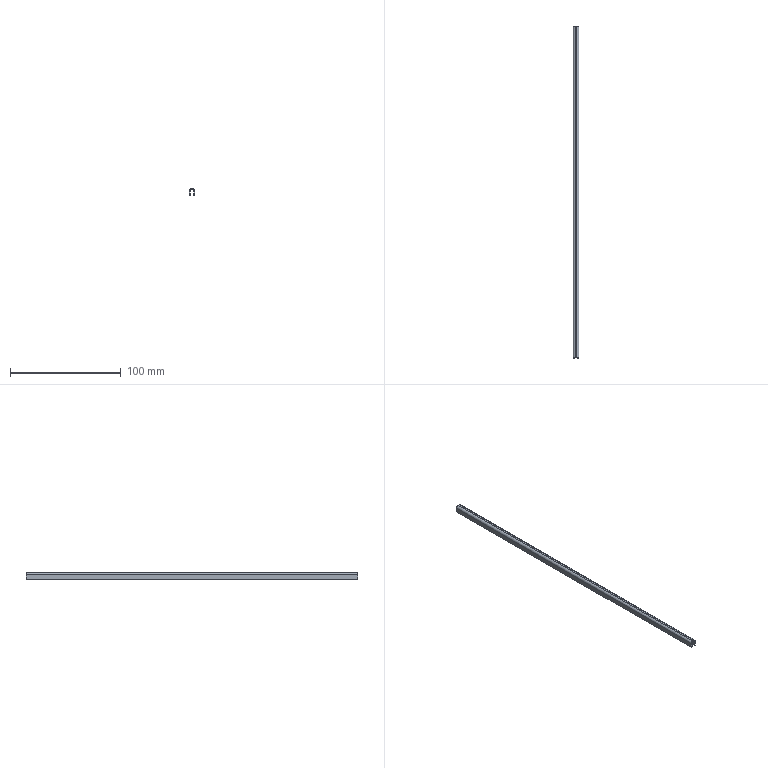Part | STEP file | Guide wheel mechanism revised.sldasm-Part-332 | 1 solid | 22 faces | box 5.4 x 300 x 6.2 mm | volume 5131 mm3 | plane 18 | cylinder 4 | commonest cylinder face diameters 1.473 x2 3.873 x2
STEP:
#1=CARTESIAN_POINT('',(-1.2,300.,-5.));
#2=VERTEX_POINT('',#1);
#3=CARTESIAN_POINT('',(-1.2,0.,-5.));
#4=VERTEX_POINT('',#3);
#5=CARTESIAN_POINT('',(-1.2,300.,-5.));
#6=DIRECTION('',(0.,-1.,0.));
#7=VECTOR('',#6,1000.);
#8=LINE('',#5,#7);
#9=EDGE_CURVE('',#2,#4,#8,.T.);
#10=ORIENTED_EDGE('',*,*,#9,.F.);
#11=CARTESIAN_POINT('',(0.,300.,-5.));
#12=VERTEX_POINT('',#11);
#13=CARTESIAN_POINT('',(598.861,300.,-5.));
#14=DIRECTION('',(-1.,0.,0.));
#15=VECTOR('',#14,1000.);
#16=LINE('',#13,#15);
#17=EDGE_CURVE('',#12,#2,#16,.T.);
#18=ORIENTED_EDGE('',*,*,#17,.F.);
#19=CARTESIAN_POINT('',(0.,0.,-5.));
#20=VERTEX_POINT('',#19);
#21=CARTESIAN_POINT('',(0.,300.,-5.));
#22=DIRECTION('',(0.,-1.,0.));
#23=VECTOR('',#22,1000.);
#24=LINE('',#21,#23);
#25=EDGE_CURVE('',#12,#20,#24,.T.);
#26=ORIENTED_EDGE('',*,*,#25,.T.);
#27=CARTESIAN_POINT('',(598.861,0.,-5.));
#28=DIRECTION('',(-1.,0.,0.));
#29=VECTOR('',#28,1000.);
#30=LINE('',#27,#29);
#31=EDGE_CURVE('',#20,#4,#30,.T.);
#32=ORIENTED_EDGE('',*,*,#31,.T.);
#33=EDGE_LOOP('',(#10,#18,#26,#32));
#34=FACE_OUTER_BOUND('',#33,.T.);
#35=CARTESIAN_POINT('',(598.861,300.,-5.));
#36=DIRECTION('',(0.,0.,-1.));
#37=DIRECTION('',(-1.,0.,0.));
#38=AXIS2_PLACEMENT_3D('',#35,#36,#37);
#39=PLANE('',#38);
#40=ADVANCED_FACE('',(#34),#39,.T.);
#41=CARTESIAN_POINT('',(-1.2,0.,-0.7366));
#42=VERTEX_POINT('',#41);
#43=CARTESIAN_POINT('',(-1.2,0.,-5.));
#44=DIRECTION('',(0.,0.,1.));
#45=VECTOR('',#44,1000.);
#46=LINE('',#43,#45);
#47=EDGE_CURVE('',#4,#42,#46,.T.);
#48=ORIENTED_EDGE('',*,*,#47,.F.);
#49=ORIENTED_EDGE('',*,*,#31,.F.);
#50=CARTESIAN_POINT('',(0.,0.,-0.7366));
#51=VERTEX_POINT('',#50);
#52=CARTESIAN_POINT('',(0.,0.,-5.));
#53=DIRECTION('',(0.,0.,1.));
#54=VECTOR('',#53,1000.);
#55=LINE('',#52,#54);
#56=EDGE_CURVE('',#20,#51,#55,.T.);
#57=ORIENTED_EDGE('',*,*,#56,.T.);
#58=CARTESIAN_POINT('',(598.861,0.,-0.7366));
#59=DIRECTION('',(-1.,0.,0.));
#60=VECTOR('',#59,1000.);
#61=LINE('',#58,#60);
#62=EDGE_CURVE('',#51,#42,#61,.T.);
#63=ORIENTED_EDGE('',*,*,#62,.T.);
#64=EDGE_LOOP('',(#48,#49,#57,#63));
#65=FACE_OUTER_BOUND('',#64,.T.);
#66=CARTESIAN_POINT('',(598.861,0.,-5.));
#67=DIRECTION('',(0.,-1.,0.));
#68=DIRECTION('',(1.,0.,0.));
#69=AXIS2_PLACEMENT_3D('',#66,#67,#68);
#70=PLANE('',#69);
#71=ADVANCED_FACE('',(#65),#70,.T.);
#72=ORIENTED_EDGE('',*,*,#47,.T.);
#73=CARTESIAN_POINT('',(-1.2,300.,-0.7366));
#74=VERTEX_POINT('',#73);
#75=CARTESIAN_POINT('',(-1.2,0.,-0.7366));
#76=DIRECTION('',(0.,1.,0.));
#77=VECTOR('',#76,1000.);
#78=LINE('',#75,#77);
#79=EDGE_CURVE('',#42,#74,#78,.T.);
#80=ORIENTED_EDGE('',*,*,#79,.T.);
#81=CARTESIAN_POINT('',(-1.2,300.,-5.));
#82=DIRECTION('',(0.,0.,1.));
#83=VECTOR('',#82,1000.);
#84=LINE('',#81,#83);
#85=EDGE_CURVE('',#2,#74,#84,.T.);
#86=ORIENTED_EDGE('',*,*,#85,.F.);
#87=ORIENTED_EDGE('',*,*,#9,.T.);
#88=EDGE_LOOP('',(#72,#80,#86,#87));
#89=FACE_OUTER_BOUND('',#88,.T.);
#90=CARTESIAN_POINT('',(-1.2,300.,-5.));
#91=DIRECTION('',(1.,0.,0.));
#92=DIRECTION('',(0.,0.,-1.));
#93=AXIS2_PLACEMENT_3D('',#90,#91,#92);
#94=PLANE('',#93);
#95=ADVANCED_FACE('',(#89),#94,.F.);
#96=ORIENTED_EDGE('',*,*,#17,.T.);
#97=ORIENTED_EDGE('',*,*,#85,.T.);
#98=CARTESIAN_POINT('',(0.,300.,-0.7366));
#99=VERTEX_POINT('',#98);
#100=CARTESIAN_POINT('',(598.861,300.,-0.7366));
#101=DIRECTION('',(-1.,0.,0.));
#102=VECTOR('',#101,1000.);
#103=LINE('',#100,#102);
#104=EDGE_CURVE('',#99,#74,#103,.T.);
#105=ORIENTED_EDGE('',*,*,#104,.F.);
#106=CARTESIAN_POINT('',(0.,300.,-5.));
#107=DIRECTION('',(0.,0.,1.));
#108=VECTOR('',#107,1000.);
#109=LINE('',#106,#108);
#110=EDGE_CURVE('',#12,#99,#109,.T.);
#111=ORIENTED_EDGE('',*,*,#110,.F.);
#112=EDGE_LOOP('',(#96,#97,#105,#111));
#113=FACE_OUTER_BOUND('',#112,.T.);
#114=CARTESIAN_POINT('',(598.861,300.,-5.));
#115=DIRECTION('',(0.,-1.,0.));
#116=DIRECTION('',(1.,0.,0.));
#117=AXIS2_PLACEMENT_3D('',#114,#115,#116);
#118=PLANE('',#117);
#119=ADVANCED_FACE('',(#113),#118,.F.);
#120=CARTESIAN_POINT('',(0.,0.,-0.7366));
#121=DIRECTION('',(0.,1.,0.));
#122=VECTOR('',#121,1000.);
#123=LINE('',#120,#122);
#124=EDGE_CURVE('',#51,#99,#123,.T.);
#125=ORIENTED_EDGE('',*,*,#124,.F.);
#126=ORIENTED_EDGE('',*,*,#56,.F.);
#127=ORIENTED_EDGE('',*,*,#25,.F.);
#128=ORIENTED_EDGE('',*,*,#110,.T.);
#129=EDGE_LOOP('',(#125,#126,#127,#128));
#130=FACE_OUTER_BOUND('',#129,.T.);
#131=CARTESIAN_POINT('',(0.,300.,-5.));
#132=DIRECTION('',(1.,0.,0.));
#133=DIRECTION('',(0.,0.,-1.));
#134=AXIS2_PLACEMENT_3D('',#131,#132,#133);
#135=PLANE('',#134);
#136=ADVANCED_FACE('',(#130),#135,.T.);
#137=CARTESIAN_POINT('',(3.,300.,-5.));
#138=VERTEX_POINT('',#137);
#139=CARTESIAN_POINT('',(4.2,300.,-5.));
#140=VERTEX_POINT('',#139);
#141=CARTESIAN_POINT('',(-595.861,300.,-5.));
#142=DIRECTION('',(1.,0.,0.));
#143=VECTOR('',#142,1000.);
#144=LINE('',#141,#143);
#145=EDGE_CURVE('',#138,#140,#144,.T.);
#146=ORIENTED_EDGE('',*,*,#145,.T.);
#147=CARTESIAN_POINT('',(4.2,0.,-5.));
#148=VERTEX_POINT('',#147);
#149=CARTESIAN_POINT('',(4.2,300.,-5.));
#150=DIRECTION('',(0.,-1.,0.));
#151=VECTOR('',#150,1000.);
#152=LINE('',#149,#151);
#153=EDGE_CURVE('',#140,#148,#152,.T.);
#154=ORIENTED_EDGE('',*,*,#153,.T.);
#155=CARTESIAN_POINT('',(3.,0.,-5.));
#156=VERTEX_POINT('',#155);
#157=CARTESIAN_POINT('',(-595.861,0.,-5.));
#158=DIRECTION('',(1.,0.,0.));
#159=VECTOR('',#158,1000.);
#160=LINE('',#157,#159);
#161=EDGE_CURVE('',#156,#148,#160,.T.);
#162=ORIENTED_EDGE('',*,*,#161,.F.);
#163=CARTESIAN_POINT('',(3.,300.,-5.));
#164=DIRECTION('',(0.,-1.,0.));
#165=VECTOR('',#164,1000.);
#166=LINE('',#163,#165);
#167=EDGE_CURVE('',#138,#156,#166,.T.);
#168=ORIENTED_EDGE('',*,*,#167,.F.);
#169=EDGE_LOOP('',(#146,#154,#162,#168));
#170=FACE_OUTER_BOUND('',#169,.T.);
#171=CARTESIAN_POINT('',(-595.861,300.,-5.));
#172=DIRECTION('',(0.,0.,1.));
#173=DIRECTION('',(1.,0.,0.));
#174=AXIS2_PLACEMENT_3D('',#171,#172,#173);
#175=PLANE('',#174);
#176=ADVANCED_FACE('',(#170),#175,.F.);
#177=CARTESIAN_POINT('',(3.,300.,-0.7366));
#178=VERTEX_POINT('',#177);
#179=CARTESIAN_POINT('',(4.2,300.,-0.7366));
#180=VERTEX_POINT('',#179);
#181=CARTESIAN_POINT('',(-595.861,300.,-0.7366));
#182=DIRECTION('',(1.,0.,0.));
#183=VECTOR('',#182,1000.);
#184=LINE('',#181,#183);
#185=EDGE_CURVE('',#178,#180,#184,.T.);
#186=ORIENTED_EDGE('',*,*,#185,.T.);
#187=CARTESIAN_POINT('',(4.2,300.,0.));
#188=DIRECTION('',(0.,0.,-1.));
#189=VECTOR('',#188,1000.);
#190=LINE('',#187,#189);
#191=EDGE_CURVE('',#180,#140,#190,.T.);
#192=ORIENTED_EDGE('',*,*,#191,.T.);
#193=ORIENTED_EDGE('',*,*,#145,.F.);
#194=CARTESIAN_POINT('',(3.,300.,0.));
#195=DIRECTION('',(0.,0.,-1.));
#196=VECTOR('',#195,1000.);
#197=LINE('',#194,#196);
#198=EDGE_CURVE('',#178,#138,#197,.T.);
#199=ORIENTED_EDGE('',*,*,#198,.F.);
#200=EDGE_LOOP('',(#186,#192,#193,#199));
#201=FACE_OUTER_BOUND('',#200,.T.);
#202=CARTESIAN_POINT('',(-595.861,300.,0.));
#203=DIRECTION('',(0.,-1.,0.));
#204=DIRECTION('',(-1.,0.,0.));
#205=AXIS2_PLACEMENT_3D('',#202,#203,#204);
#206=PLANE('',#205);
#207=ADVANCED_FACE('',(#201),#206,.F.);
#208=ORIENTED_EDGE('',*,*,#191,.F.);
#209=CARTESIAN_POINT('',(4.2,0.,-0.7366));
#210=VERTEX_POINT('',#209);
#211=CARTESIAN_POINT('',(4.2,300.,-0.7366));
#212=DIRECTION('',(0.,-1.,0.));
#213=VECTOR('',#212,1000.);
#214=LINE('',#211,#213);
#215=EDGE_CURVE('',#180,#210,#214,.T.);
#216=ORIENTED_EDGE('',*,*,#215,.T.);
#217=CARTESIAN_POINT('',(4.2,0.,0.));
#218=DIRECTION('',(0.,0.,-1.));
#219=VECTOR('',#218,1000.);
#220=LINE('',#217,#219);
#221=EDGE_CURVE('',#210,#148,#220,.T.);
#222=ORIENTED_EDGE('',*,*,#221,.T.);
#223=ORIENTED_EDGE('',*,*,#153,.F.);
#224=EDGE_LOOP('',(#208,#216,#222,#223));
#225=FACE_OUTER_BOUND('',#224,.T.);
#226=CARTESIAN_POINT('',(4.2,300.,0.));
#227=DIRECTION('',(-1.,0.,0.));
#228=DIRECTION('',(0.,0.,1.));
#229=AXIS2_PLACEMENT_3D('',#226,#227,#228);
#230=PLANE('',#229);
#231=ADVANCED_FACE('',(#225),#230,.F.);
#232=ORIENTED_EDGE('',*,*,#221,.F.);
#233=CARTESIAN_POINT('',(3.,0.,-0.7366));
#234=VERTEX_POINT('',#233);
#235=CARTESIAN_POINT('',(-595.861,0.,-0.7366));
#236=DIRECTION('',(1.,0.,0.));
#237=VECTOR('',#236,1000.);
#238=LINE('',#235,#237);
#239=EDGE_CURVE('',#234,#210,#238,.T.);
#240=ORIENTED_EDGE('',*,*,#239,.F.);
#241=CARTESIAN_POINT('',(3.,0.,0.));
#242=DIRECTION('',(0.,0.,-1.));
#243=VECTOR('',#242,1000.);
#244=LINE('',#241,#243);
#245=EDGE_CURVE('',#234,#156,#244,.T.);
#246=ORIENTED_EDGE('',*,*,#245,.T.);
#247=ORIENTED_EDGE('',*,*,#161,.T.);
#248=EDGE_LOOP('',(#232,#240,#246,#247));
#249=FACE_OUTER_BOUND('',#248,.T.);
#250=CARTESIAN_POINT('',(-595.861,0.,0.));
#251=DIRECTION('',(0.,-1.,0.));
#252=DIRECTION('',(-1.,0.,0.));
#253=AXIS2_PLACEMENT_3D('',#250,#251,#252);
#254=PLANE('',#253);
#255=ADVANCED_FACE('',(#249),#254,.T.);
#256=CARTESIAN_POINT('',(3.,300.,-0.7366));
#257=DIRECTION('',(0.,-1.,0.));
#258=VECTOR('',#257,1000.);
#259=LINE('',#256,#258);
#260=EDGE_CURVE('',#178,#234,#259,.T.);
#261=ORIENTED_EDGE('',*,*,#260,.F.);
#262=ORIENTED_EDGE('',*,*,#198,.T.);
#263=ORIENTED_EDGE('',*,*,#167,.T.);
#264=ORIENTED_EDGE('',*,*,#245,.F.);
#265=EDGE_LOOP('',(#261,#262,#263,#264));
#266=FACE_OUTER_BOUND('',#265,.T.);
#267=CARTESIAN_POINT('',(3.,300.,0.));
#268=DIRECTION('',(-1.,0.,0.));
#269=DIRECTION('',(0.,0.,1.));
#270=AXIS2_PLACEMENT_3D('',#267,#268,#269);
#271=PLANE('',#270);
#272=ADVANCED_FACE('',(#266),#271,.T.);
#273=CARTESIAN_POINT('',(0.7366,0.,1.2));
#274=VERTEX_POINT('',#273);
#275=CARTESIAN_POINT('',(2.263,0.,1.2));
#276=VERTEX_POINT('',#275);
#277=CARTESIAN_POINT('',(0.,0.,1.2));
#278=DIRECTION('',(1.,0.,0.));
#279=VECTOR('',#278,1000.);
#280=LINE('',#277,#279);
#281=EDGE_CURVE('',#274,#276,#280,.T.);
#282=ORIENTED_EDGE('',*,*,#281,.F.);
#283=CARTESIAN_POINT('',(0.7366,0.,0.));
#284=VERTEX_POINT('',#283);
#285=CARTESIAN_POINT('',(0.7366,0.,-598.808));
#286=DIRECTION('',(0.,0.,1.));
#287=VECTOR('',#286,1000.);
#288=LINE('',#285,#287);
#289=EDGE_CURVE('',#284,#274,#288,.T.);
#290=ORIENTED_EDGE('',*,*,#289,.F.);
#291=CARTESIAN_POINT('',(2.263,0.,0.));
#292=VERTEX_POINT('',#291);
#293=CARTESIAN_POINT('',(0.,0.,0.));
#294=DIRECTION('',(1.,0.,0.));
#295=VECTOR('',#294,1000.);
#296=LINE('',#293,#295);
#297=EDGE_CURVE('',#284,#292,#296,.T.);
#298=ORIENTED_EDGE('',*,*,#297,.T.);
#299=CARTESIAN_POINT('',(2.263,0.,-598.808));
#300=DIRECTION('',(0.,0.,1.));
#301=VECTOR('',#300,1000.);
#302=LINE('',#299,#301);
#303=EDGE_CURVE('',#292,#276,#302,.T.);
#304=ORIENTED_EDGE('',*,*,#303,.T.);
#305=EDGE_LOOP('',(#282,#290,#298,#304));
#306=FACE_OUTER_BOUND('',#305,.T.);
#307=CARTESIAN_POINT('',(0.,0.,-598.808));
#308=DIRECTION('',(0.,-1.,0.));
#309=DIRECTION('',(0.,0.,-1.));
#310=AXIS2_PLACEMENT_3D('',#307,#308,#309);
#311=PLANE('',#310);
#312=ADVANCED_FACE('',(#306),#311,.T.);
#313=CARTESIAN_POINT('',(0.7366,300.,0.));
#314=VERTEX_POINT('',#313);
#315=CARTESIAN_POINT('',(0.7366,300.,1.2));
#316=VERTEX_POINT('',#315);
#317=CARTESIAN_POINT('',(0.7366,300.,-598.808));
#318=DIRECTION('',(0.,0.,1.));
#319=VECTOR('',#318,1000.);
#320=LINE('',#317,#319);
#321=EDGE_CURVE('',#314,#316,#320,.T.);
#322=ORIENTED_EDGE('',*,*,#321,.T.);
#323=CARTESIAN_POINT('',(2.263,300.,1.2));
#324=VERTEX_POINT('',#323);
#325=CARTESIAN_POINT('',(0.,300.,1.2));
#326=DIRECTION('',(1.,0.,0.));
#327=VECTOR('',#326,1000.);
#328=LINE('',#325,#327);
#329=EDGE_CURVE('',#316,#324,#328,.T.);
#330=ORIENTED_EDGE('',*,*,#329,.T.);
#331=CARTESIAN_POINT('',(2.263,300.,0.));
#332=VERTEX_POINT('',#331);
#333=CARTESIAN_POINT('',(2.263,300.,-598.808));
#334=DIRECTION('',(0.,0.,1.));
#335=VECTOR('',#334,1000.);
#336=LINE('',#333,#335);
#337=EDGE_CURVE('',#332,#324,#336,.T.);
#338=ORIENTED_EDGE('',*,*,#337,.F.);
#339=CARTESIAN_POINT('',(0.,300.,0.));
#340=DIRECTION('',(1.,0.,0.));
#341=VECTOR('',#340,1000.);
#342=LINE('',#339,#341);
#343=EDGE_CURVE('',#314,#332,#342,.T.);
#344=ORIENTED_EDGE('',*,*,#343,.F.);
#345=EDGE_LOOP('',(#322,#330,#338,#344));
#346=FACE_OUTER_BOUND('',#345,.T.);
#347=CARTESIAN_POINT('',(0.,300.,-598.808));
#348=DIRECTION('',(0.,-1.,0.));
#349=DIRECTION('',(0.,0.,-1.));
#350=AXIS2_PLACEMENT_3D('',#347,#348,#349);
#351=PLANE('',#350);
#352=ADVANCED_FACE('',(#346),#351,.F.);
#353=ORIENTED_EDGE('',*,*,#297,.F.);
#354=CARTESIAN_POINT('',(0.7366,0.,0.));
#355=DIRECTION('',(0.,1.,0.));
#356=VECTOR('',#355,1000.);
#357=LINE('',#354,#356);
#358=EDGE_CURVE('',#284,#314,#357,.T.);
#359=ORIENTED_EDGE('',*,*,#358,.T.);
#360=ORIENTED_EDGE('',*,*,#343,.T.);
#361=CARTESIAN_POINT('',(2.263,300.,0.));
#362=DIRECTION('',(0.,-1.,0.));
#363=VECTOR('',#362,1000.);
#364=LINE('',#361,#363);
#365=EDGE_CURVE('',#332,#292,#364,.T.);
#366=ORIENTED_EDGE('',*,*,#365,.T.);
#367=EDGE_LOOP('',(#353,#359,#360,#366));
#368=FACE_OUTER_BOUND('',#367,.T.);
#369=CARTESIAN_POINT('',(0.,300.,0.));
#370=DIRECTION('',(0.,0.,-1.));
#371=DIRECTION('',(-1.,0.,0.));
#372=AXIS2_PLACEMENT_3D('',#369,#370,#371);
#373=PLANE('',#372);
#374=ADVANCED_FACE('',(#368),#373,.T.);
#375=CARTESIAN_POINT('',(0.7366,0.,1.2));
#376=DIRECTION('',(0.,1.,0.));
#377=VECTOR('',#376,1000.);
#378=LINE('',#375,#377);
#379=EDGE_CURVE('',#274,#316,#378,.T.);
#380=ORIENTED_EDGE('',*,*,#379,.F.);
#381=ORIENTED_EDGE('',*,*,#281,.T.);
#382=CARTESIAN_POINT('',(2.263,300.,1.2));
#383=DIRECTION('',(0.,-1.,0.));
#384=VECTOR('',#383,1000.);
#385=LINE('',#382,#384);
#386=EDGE_CURVE('',#324,#276,#385,.T.);
#387=ORIENTED_EDGE('',*,*,#386,.F.);
#388=ORIENTED_EDGE('',*,*,#329,.F.);
#389=EDGE_LOOP('',(#380,#381,#387,#388));
#390=FACE_OUTER_BOUND('',#389,.T.);
#391=CARTESIAN_POINT('',(0.,300.,1.2));
#392=DIRECTION('',(0.,0.,-1.));
#393=DIRECTION('',(-1.,0.,0.));
#394=AXIS2_PLACEMENT_3D('',#391,#392,#393);
#395=PLANE('',#394);
#396=ADVANCED_FACE('',(#390),#395,.F.);
#397=ORIENTED_EDGE('',*,*,#303,.F.);
#398=CARTESIAN_POINT('',(2.263,0.,-0.7366));
#399=DIRECTION('',(0.,1.,0.));
#400=DIRECTION('',(0.,0.,-1.));
#401=AXIS2_PLACEMENT_3D('',#398,#399,#400);
#402=CIRCLE('',#401,0.7366);
#403=EDGE_CURVE('',#292,#234,#402,.T.);
#404=ORIENTED_EDGE('',*,*,#403,.T.);
#405=ORIENTED_EDGE('',*,*,#239,.T.);
#406=CARTESIAN_POINT('',(2.263,0.,-0.7366));
#407=DIRECTION('',(0.,1.,0.));
#408=DIRECTION('',(0.,0.,-1.));
#409=AXIS2_PLACEMENT_3D('',#406,#407,#408);
#410=CIRCLE('',#409,1.937);
#411=EDGE_CURVE('',#276,#210,#410,.T.);
#412=ORIENTED_EDGE('',*,*,#411,.F.);
#413=EDGE_LOOP('',(#397,#404,#405,#412));
#414=FACE_OUTER_BOUND('',#413,.T.);
#415=CARTESIAN_POINT('',(2.263,0.,-0.7366));
#416=DIRECTION('',(0.,-1.,0.));
#417=DIRECTION('',(0.,0.,-1.));
#418=AXIS2_PLACEMENT_3D('',#415,#416,#417);
#419=PLANE('',#418);
#420=ADVANCED_FACE('',(#414),#419,.T.);
#421=ORIENTED_EDGE('',*,*,#185,.F.);
#422=CARTESIAN_POINT('',(2.263,300.,-0.7366));
#423=DIRECTION('',(0.,-1.,0.));
#424=DIRECTION('',(0.,0.,-1.));
#425=AXIS2_PLACEMENT_3D('',#422,#423,#424);
#426=CIRCLE('',#425,0.7366);
#427=EDGE_CURVE('',#178,#332,#426,.T.);
#428=ORIENTED_EDGE('',*,*,#427,.T.);
#429=ORIENTED_EDGE('',*,*,#337,.T.);
#430=CARTESIAN_POINT('',(2.263,300.,-0.7366));
#431=DIRECTION('',(0.,-1.,0.));
#432=DIRECTION('',(0.,0.,-1.));
#433=AXIS2_PLACEMENT_3D('',#430,#431,#432);
#434=CIRCLE('',#433,1.937);
#435=EDGE_CURVE('',#180,#324,#434,.T.);
#436=ORIENTED_EDGE('',*,*,#435,.F.);
#437=EDGE_LOOP('',(#421,#428,#429,#436));
#438=FACE_OUTER_BOUND('',#437,.T.);
#439=CARTESIAN_POINT('',(2.263,300.,-0.7366));
#440=DIRECTION('',(0.,1.,0.));
#441=DIRECTION('',(0.,0.,1.));
#442=AXIS2_PLACEMENT_3D('',#439,#440,#441);
#443=PLANE('',#442);
#444=ADVANCED_FACE('',(#438),#443,.T.);
#445=ORIENTED_EDGE('',*,*,#435,.T.);
#446=ORIENTED_EDGE('',*,*,#386,.T.);
#447=ORIENTED_EDGE('',*,*,#411,.T.);
#448=ORIENTED_EDGE('',*,*,#215,.F.);
#449=EDGE_LOOP('',(#445,#446,#447,#448));
#450=FACE_OUTER_BOUND('',#449,.T.);
#451=CARTESIAN_POINT('',(2.263,600.341,-0.7366));
#452=DIRECTION('',(0.,-1.,0.));
#453=DIRECTION('',(0.,0.,-1.));
#454=AXIS2_PLACEMENT_3D('',#451,#452,#453);
#455=CYLINDRICAL_SURFACE('',#454,1.937);
#456=ADVANCED_FACE('',(#450),#455,.T.);
#457=ORIENTED_EDGE('',*,*,#427,.F.);
#458=ORIENTED_EDGE('',*,*,#260,.T.);
#459=ORIENTED_EDGE('',*,*,#403,.F.);
#460=ORIENTED_EDGE('',*,*,#365,.F.);
#461=EDGE_LOOP('',(#457,#458,#459,#460));
#462=FACE_OUTER_BOUND('',#461,.T.);
#463=CARTESIAN_POINT('',(2.263,600.341,-0.7366));
#464=DIRECTION('',(0.,-1.,0.));
#465=DIRECTION('',(0.,0.,-1.));
#466=AXIS2_PLACEMENT_3D('',#463,#464,#465);
#467=CYLINDRICAL_SURFACE('',#466,0.7366);
#468=ADVANCED_FACE('',(#462),#467,.F.);
#469=ORIENTED_EDGE('',*,*,#321,.F.);
#470=CARTESIAN_POINT('',(0.7366,300.,-0.7366));
#471=DIRECTION('',(0.,-1.,0.));
#472=DIRECTION('',(0.,0.,1.));
#473=AXIS2_PLACEMENT_3D('',#470,#471,#472);
#474=CIRCLE('',#473,0.7366);
#475=EDGE_CURVE('',#314,#99,#474,.T.);
#476=ORIENTED_EDGE('',*,*,#475,.T.);
#477=ORIENTED_EDGE('',*,*,#104,.T.);
#478=CARTESIAN_POINT('',(0.7366,300.,-0.7366));
#479=DIRECTION('',(0.,-1.,0.));
#480=DIRECTION('',(0.,0.,1.));
#481=AXIS2_PLACEMENT_3D('',#478,#479,#480);
#482=CIRCLE('',#481,1.937);
#483=EDGE_CURVE('',#316,#74,#482,.T.);
#484=ORIENTED_EDGE('',*,*,#483,.F.);
#485=EDGE_LOOP('',(#469,#476,#477,#484));
#486=FACE_OUTER_BOUND('',#485,.T.);
#487=CARTESIAN_POINT('',(0.7366,300.,-0.7366));
#488=DIRECTION('',(0.,1.,0.));
#489=DIRECTION('',(0.,0.,1.));
#490=AXIS2_PLACEMENT_3D('',#487,#488,#489);
#491=PLANE('',#490);
#492=ADVANCED_FACE('',(#486),#491,.T.);
#493=ORIENTED_EDGE('',*,*,#62,.F.);
#494=CARTESIAN_POINT('',(0.7366,0.,-0.7366));
#495=DIRECTION('',(0.,1.,0.));
#496=DIRECTION('',(0.,0.,1.));
#497=AXIS2_PLACEMENT_3D('',#494,#495,#496);
#498=CIRCLE('',#497,0.7366);
#499=EDGE_CURVE('',#51,#284,#498,.T.);
#500=ORIENTED_EDGE('',*,*,#499,.T.);
#501=ORIENTED_EDGE('',*,*,#289,.T.);
#502=CARTESIAN_POINT('',(0.7366,0.,-0.7366));
#503=DIRECTION('',(0.,1.,0.));
#504=DIRECTION('',(0.,0.,1.));
#505=AXIS2_PLACEMENT_3D('',#502,#503,#504);
#506=CIRCLE('',#505,1.937);
#507=EDGE_CURVE('',#42,#274,#506,.T.);
#508=ORIENTED_EDGE('',*,*,#507,.F.);
#509=EDGE_LOOP('',(#493,#500,#501,#508));
#510=FACE_OUTER_BOUND('',#509,.T.);
#511=CARTESIAN_POINT('',(0.7366,0.,-0.7366));
#512=DIRECTION('',(0.,-1.,0.));
#513=DIRECTION('',(0.,0.,-1.));
#514=AXIS2_PLACEMENT_3D('',#511,#512,#513);
#515=PLANE('',#514);
#516=ADVANCED_FACE('',(#510),#515,.T.);
#517=ORIENTED_EDGE('',*,*,#507,.T.);
#518=ORIENTED_EDGE('',*,*,#379,.T.);
#519=ORIENTED_EDGE('',*,*,#483,.T.);
#520=ORIENTED_EDGE('',*,*,#79,.F.);
#521=EDGE_LOOP('',(#517,#518,#519,#520));
#522=FACE_OUTER_BOUND('',#521,.T.);
#523=CARTESIAN_POINT('',(0.7366,-300.225,-0.7366));
#524=DIRECTION('',(0.,1.,0.));
#525=DIRECTION('',(0.,0.,1.));
#526=AXIS2_PLACEMENT_3D('',#523,#524,#525);
#527=CYLINDRICAL_SURFACE('',#526,1.937);
#528=ADVANCED_FACE('',(#522),#527,.T.);
#529=ORIENTED_EDGE('',*,*,#499,.F.);
#530=ORIENTED_EDGE('',*,*,#124,.T.);
#531=ORIENTED_EDGE('',*,*,#475,.F.);
#532=ORIENTED_EDGE('',*,*,#358,.F.);
#533=EDGE_LOOP('',(#529,#530,#531,#532));
#534=FACE_OUTER_BOUND('',#533,.T.);
#535=CARTESIAN_POINT('',(0.7366,-300.225,-0.7366));
#536=DIRECTION('',(0.,1.,0.));
#537=DIRECTION('',(0.,0.,1.));
#538=AXIS2_PLACEMENT_3D('',#535,#536,#537);
#539=CYLINDRICAL_SURFACE('',#538,0.7366);
#540=ADVANCED_FACE('',(#534),#539,.F.);
#541=CLOSED_SHELL('',(#40,#71,#95,#119,#136,#176,#207,#231,#255,#272,#312,#352,#374,#396,#420,#444,#456,#468,#492,#516,#528,#540));
#542=MANIFOLD_SOLID_BREP('',#541);
#543=CARTESIAN_POINT('',(0.,0.,0.));
#544=DIRECTION('',(0.,0.,1.));
#545=DIRECTION('',(1.,0.,0.));
#546=AXIS2_PLACEMENT_3D('',#543,#544,#545);
#547=(LENGTH_UNIT()NAMED_UNIT(*)SI_UNIT(.MILLI.,.METRE.));
#548=UNCERTAINTY_MEASURE_WITH_UNIT(LENGTH_MEASURE(0.00001),#547,'','');
#549=(NAMED_UNIT(*)PLANE_ANGLE_UNIT()SI_UNIT($,.RADIAN.));
#550=(NAMED_UNIT(*)SI_UNIT($,.STERADIAN.)SOLID_ANGLE_UNIT());
#551=(GEOMETRIC_REPRESENTATION_CONTEXT(3)GLOBAL_UNCERTAINTY_ASSIGNED_CONTEXT((#548))GLOBAL_UNIT_ASSIGNED_CONTEXT((#547,#549,#550))REPRESENTATION_CONTEXT('',''));
#552=ADVANCED_BREP_SHAPE_REPRESENTATION('',(#542,#546),#551);